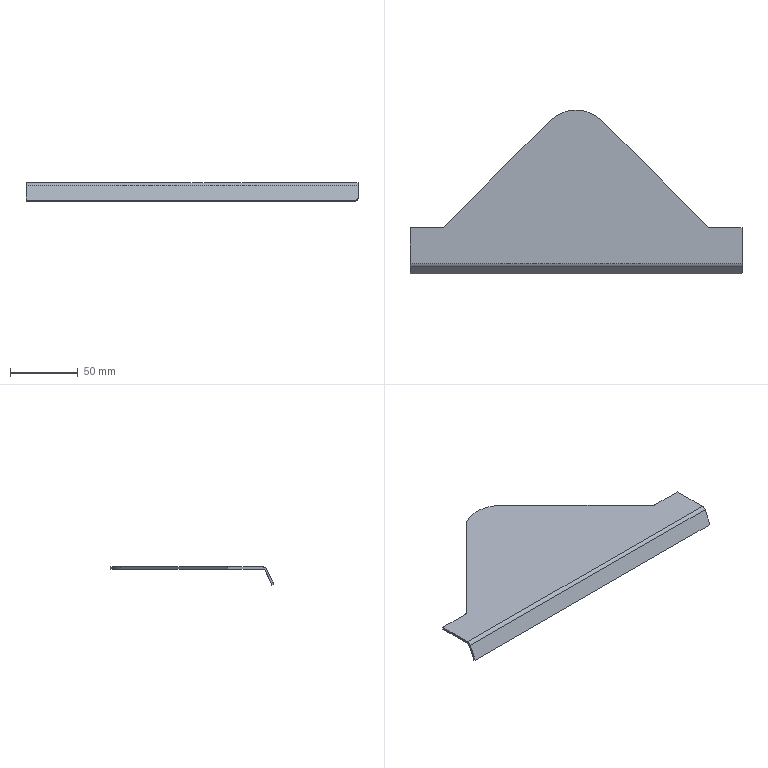Part | STEP file | Guard wheel drive wer2 part2 | 1 solid | 21 faces | box 245 x 120.904 x 13.322 mm | volume 29188 mm3 | plane 15 | cylinder 6 | commonest cylinder face diameters 3 x3 4 x1 6 x1 54 x1
STEP:
#1=CARTESIAN_POINT('',(0.,0.,0.));
#2=DIRECTION('',(0.,0.,1.));
#3=DIRECTION('',(1.,0.,0.));
#4=AXIS2_PLACEMENT_3D('',#1,#2,#3);
#5=CARTESIAN_POINT('',(221.305,-31.558,-9.376));
#6=VERTEX_POINT('',#5);
#7=CARTESIAN_POINT('',(219.305,-32.404,-11.188));
#8=VERTEX_POINT('',#7);
#9=CARTESIAN_POINT('',(219.305,-31.558,-9.376));
#10=DIRECTION('',(0.,0.9063,-0.4226));
#11=DIRECTION('',(0.7071,-0.2988,-0.6409));
#12=AXIS2_PLACEMENT_3D('',#9,#10,#11);
#13=CIRCLE('',#12,2.);
#14=CARTESIAN_POINT('',(219.305,-30.199,-10.01));
#15=DIRECTION('',(0.,-0.9063,0.4226));
#16=DIRECTION('',(0.7071,-0.2988,-0.6409));
#17=AXIS2_PLACEMENT_3D('',#14,#15,#16);
#18=CYLINDRICAL_SURFACE('',#17,2.);
#19=CARTESIAN_POINT('',(12.566,1.5));
#20=DIRECTION('',(-1.,0.));
#21=VECTOR('',#20,1.);
#22=LINE('',#19,#21);
#23=(GEOMETRIC_REPRESENTATION_CONTEXT(2)PARAMETRIC_REPRESENTATION_CONTEXT()REPRESENTATION_CONTEXT('',''));
#24=DEFINITIONAL_REPRESENTATION('',(#22),#23);
#25=PCURVE('',#18,#24);
#26=CARTESIAN_POINT('',(98.805,-29.331,-4.6));
#27=DIRECTION('',(0.,-0.9063,0.4226));
#28=DIRECTION('',(1.,0.,0.));
#29=AXIS2_PLACEMENT_3D('',#26,#27,#28);
#30=PLANE('',#29);
#31=CARTESIAN_POINT('',(121.914,-6.684));
#32=CARTESIAN_POINT('',(119.465,-9.133));
#33=CARTESIAN_POINT('',(118.568,-5.787));
#34=CARTESIAN_POINT('',(117.672,-2.441));
#35=CARTESIAN_POINT('',(121.018,-3.338));
#36=CARTESIAN_POINT('',(124.364,-4.234));
#37=CARTESIAN_POINT('',(121.914,-6.684));
#38=(BOUNDED_CURVE()B_SPLINE_CURVE(2,(#31,#32,#33,#34,#35,#36,#37),.UNSPECIFIED.,.T.,.F.)B_SPLINE_CURVE_WITH_KNOTS((1,2,2,2,2,1),(-2.094,0.,2.094,4.189,6.283,8.378),.UNSPECIFIED.)CURVE()GEOMETRIC_REPRESENTATION_ITEM()RATIONAL_B_SPLINE_CURVE((1.,0.5,1.,0.5,1.,0.5,1.))REPRESENTATION_ITEM(''));
#39=(GEOMETRIC_REPRESENTATION_CONTEXT(2)PARAMETRIC_REPRESENTATION_CONTEXT()REPRESENTATION_CONTEXT('',''));
#40=DEFINITIONAL_REPRESENTATION('',(#38),#39);
#41=PCURVE('',#30,#40);
#42=SURFACE_CURVE('',#13,(#25,#41),.PCURVE_S1.);
#43=EDGE_CURVE('',#6,#8,#42,.T.);
#44=ORIENTED_EDGE('',*,*,#43,.T.);
#45=CARTESIAN_POINT('',(219.305,-31.044,-11.822));
#46=VERTEX_POINT('',#45);
#47=CARTESIAN_POINT('',(219.305,-31.044,-11.822));
#48=DIRECTION('',(0.,0.9063,-0.4226));
#49=VECTOR('',#48,1.);
#50=LINE('',#47,#49);
#51=CARTESIAN_POINT('',(5.498,0.));
#52=DIRECTION('',(0.,-1.));
#53=VECTOR('',#52,1.);
#54=LINE('',#51,#53);
#55=(GEOMETRIC_REPRESENTATION_CONTEXT(2)PARAMETRIC_REPRESENTATION_CONTEXT()REPRESENTATION_CONTEXT('',''));
#56=DEFINITIONAL_REPRESENTATION('',(#54),#55);
#57=PCURVE('',#18,#56);
#58=CARTESIAN_POINT('',(221.305,-31.044,-11.822));
#59=DIRECTION('',(0.,-0.4226,-0.9063));
#60=DIRECTION('',(0.,0.9063,-0.4226));
#61=AXIS2_PLACEMENT_3D('',#58,#59,#60);
#62=PLANE('',#61);
#63=CARTESIAN_POINT('',(0.,-2.));
#64=DIRECTION('',(1.,0.));
#65=VECTOR('',#64,1.);
#66=LINE('',#63,#65);
#67=(GEOMETRIC_REPRESENTATION_CONTEXT(2)PARAMETRIC_REPRESENTATION_CONTEXT()REPRESENTATION_CONTEXT('',''));
#68=DEFINITIONAL_REPRESENTATION('',(#66),#67);
#69=PCURVE('',#62,#68);
#70=SURFACE_CURVE('',#50,(#57,#69),.PCURVE_S1.);
#71=EDGE_CURVE('',#8,#46,#70,.T.);
#72=ORIENTED_EDGE('',*,*,#71,.T.);
#73=CARTESIAN_POINT('',(221.305,-30.199,-10.01));
#74=VERTEX_POINT('',#73);
#75=CARTESIAN_POINT('',(219.305,-30.199,-10.01));
#76=DIRECTION('',(0.,-0.9063,0.4226));
#77=DIRECTION('',(0.7071,-0.2988,-0.6409));
#78=AXIS2_PLACEMENT_3D('',#75,#76,#77);
#79=CIRCLE('',#78,2.);
#80=CARTESIAN_POINT('',(0.,0.));
#81=DIRECTION('',(1.,0.));
#82=VECTOR('',#81,1.);
#83=LINE('',#80,#82);
#84=(GEOMETRIC_REPRESENTATION_CONTEXT(2)PARAMETRIC_REPRESENTATION_CONTEXT()REPRESENTATION_CONTEXT('',''));
#85=DEFINITIONAL_REPRESENTATION('',(#83),#84);
#86=PCURVE('',#18,#85);
#87=CARTESIAN_POINT('',(98.805,-27.972,-5.234));
#88=DIRECTION('',(0.,-0.9063,0.4226));
#89=DIRECTION('',(1.,0.,0.));
#90=AXIS2_PLACEMENT_3D('',#87,#88,#89);
#91=PLANE('',#90);
#92=CARTESIAN_POINT('',(120.5,-5.27));
#93=DIRECTION('',(0.7071,-0.7071));
#94=AXIS2_PLACEMENT_2D('',#92,#93);
#95=CIRCLE('',#94,2.);
#96=(GEOMETRIC_REPRESENTATION_CONTEXT(2)PARAMETRIC_REPRESENTATION_CONTEXT()REPRESENTATION_CONTEXT('',''));
#97=DEFINITIONAL_REPRESENTATION('',(#95),#96);
#98=PCURVE('',#91,#97);
#99=SURFACE_CURVE('',#79,(#86,#98),.PCURVE_S1.);
#100=EDGE_CURVE('',#46,#74,#99,.T.);
#101=ORIENTED_EDGE('',*,*,#100,.T.);
#102=CARTESIAN_POINT('',(221.305,-30.199,-10.01));
#103=DIRECTION('',(0.,-0.9063,0.4226));
#104=VECTOR('',#103,1.);
#105=LINE('',#102,#104);
#106=CARTESIAN_POINT('',(7.069,0.));
#107=DIRECTION('',(0.,1.));
#108=VECTOR('',#107,1.);
#109=LINE('',#106,#108);
#110=(GEOMETRIC_REPRESENTATION_CONTEXT(2)PARAMETRIC_REPRESENTATION_CONTEXT()REPRESENTATION_CONTEXT('',''));
#111=DEFINITIONAL_REPRESENTATION('',(#109),#110);
#112=PCURVE('',#18,#111);
#113=CARTESIAN_POINT('',(221.305,-25.935,-0.8661));
#114=DIRECTION('',(1.,0.,0.));
#115=DIRECTION('',(0.,0.9063,-0.4226));
#116=AXIS2_PLACEMENT_3D('',#113,#114,#115);
#117=PLANE('',#116);
#118=CARTESIAN_POINT('',(0.,-10.089));
#119=DIRECTION('',(-1.,0.));
#120=VECTOR('',#119,1.);
#121=LINE('',#118,#120);
#122=(GEOMETRIC_REPRESENTATION_CONTEXT(2)PARAMETRIC_REPRESENTATION_CONTEXT()REPRESENTATION_CONTEXT('',''));
#123=DEFINITIONAL_REPRESENTATION('',(#121),#122);
#124=PCURVE('',#117,#123);
#125=SURFACE_CURVE('',#105,(#112,#124),.PCURVE_S1.);
#126=EDGE_CURVE('',#74,#6,#125,.T.);
#127=ORIENTED_EDGE('',*,*,#126,.T.);
#128=EDGE_LOOP('',(#44,#72,#101,#127));
#129=FACE_BOUND('',#128,.T.);
#130=ADVANCED_FACE('',(#129),#18,.T.);
#131=ORIENTED_EDGE('',*,*,#126,.F.);
#132=CARTESIAN_POINT('',(221.305,-25.935,-0.8661));
#133=VERTEX_POINT('',#132);
#134=CARTESIAN_POINT('',(221.305,-23.067,5.284));
#135=DIRECTION('',(0.,0.4226,0.9063));
#136=VECTOR('',#135,1.);
#137=LINE('',#134,#136);
#138=CARTESIAN_POINT('',(0.,6.786));
#139=DIRECTION('',(0.,1.));
#140=VECTOR('',#139,1.);
#141=LINE('',#138,#140);
#142=(GEOMETRIC_REPRESENTATION_CONTEXT(2)PARAMETRIC_REPRESENTATION_CONTEXT()REPRESENTATION_CONTEXT('',''));
#143=DEFINITIONAL_REPRESENTATION('',(#141),#142);
#144=PCURVE('',#117,#143);
#145=CARTESIAN_POINT('',(122.5,11.605));
#146=DIRECTION('',(0.,1.));
#147=VECTOR('',#146,1.);
#148=LINE('',#145,#147);
#149=(GEOMETRIC_REPRESENTATION_CONTEXT(2)PARAMETRIC_REPRESENTATION_CONTEXT()REPRESENTATION_CONTEXT('',''));
#150=DEFINITIONAL_REPRESENTATION('',(#148),#149);
#151=PCURVE('',#91,#150);
#152=SURFACE_CURVE('',#137,(#144,#151),.PCURVE_S1.);
#153=EDGE_CURVE('',#74,#133,#152,.T.);
#154=ORIENTED_EDGE('',*,*,#153,.T.);
#155=CARTESIAN_POINT('',(221.305,-27.295,-0.2321));
#156=VERTEX_POINT('',#155);
#157=CARTESIAN_POINT('',(221.305,-26.234,-0.7266));
#158=DIRECTION('',(0.,-0.9063,0.4226));
#159=VECTOR('',#158,1.);
#160=LINE('',#157,#159);
#161=CARTESIAN_POINT('',(-0.33,0.));
#162=DIRECTION('',(-1.,0.));
#163=VECTOR('',#162,1.);
#164=LINE('',#161,#163);
#165=(GEOMETRIC_REPRESENTATION_CONTEXT(2)PARAMETRIC_REPRESENTATION_CONTEXT()REPRESENTATION_CONTEXT('',''));
#166=DEFINITIONAL_REPRESENTATION('',(#164),#165);
#167=PCURVE('',#117,#166);
#168=CARTESIAN_POINT('',(221.305,-25.935,-0.8661));
#169=DIRECTION('',(1.,0.,0.));
#170=DIRECTION('',(0.,0.,-1.));
#171=AXIS2_PLACEMENT_3D('',#168,#169,#170);
#172=PLANE('',#171);
#173=CARTESIAN_POINT('',(-0.1395,-0.2991));
#174=DIRECTION('',(-0.4226,-0.9063));
#175=VECTOR('',#174,1.);
#176=LINE('',#173,#175);
#177=(GEOMETRIC_REPRESENTATION_CONTEXT(2)PARAMETRIC_REPRESENTATION_CONTEXT()REPRESENTATION_CONTEXT('',''));
#178=DEFINITIONAL_REPRESENTATION('',(#176),#177);
#179=PCURVE('',#172,#178);
#180=SURFACE_CURVE('',#160,(#167,#179),.PCURVE_S1.);
#181=EDGE_CURVE('',#133,#156,#180,.T.);
#182=ORIENTED_EDGE('',*,*,#181,.T.);
#183=CARTESIAN_POINT('',(221.305,-27.295,-0.2321));
#184=DIRECTION('',(0.,-0.4226,-0.9063));
#185=VECTOR('',#184,1.);
#186=LINE('',#183,#185);
#187=CARTESIAN_POINT('',(-1.5,0.));
#188=DIRECTION('',(0.,-1.));
#189=VECTOR('',#188,1.);
#190=LINE('',#187,#189);
#191=(GEOMETRIC_REPRESENTATION_CONTEXT(2)PARAMETRIC_REPRESENTATION_CONTEXT()REPRESENTATION_CONTEXT('',''));
#192=DEFINITIONAL_REPRESENTATION('',(#190),#191);
#193=PCURVE('',#117,#192);
#194=CARTESIAN_POINT('',(122.5,4.819));
#195=DIRECTION('',(0.,-1.));
#196=VECTOR('',#195,1.);
#197=LINE('',#194,#196);
#198=(GEOMETRIC_REPRESENTATION_CONTEXT(2)PARAMETRIC_REPRESENTATION_CONTEXT()REPRESENTATION_CONTEXT('',''));
#199=DEFINITIONAL_REPRESENTATION('',(#197),#198);
#200=PCURVE('',#30,#199);
#201=SURFACE_CURVE('',#186,(#193,#200),.PCURVE_S1.);
#202=EDGE_CURVE('',#156,#6,#201,.T.);
#203=ORIENTED_EDGE('',*,*,#202,.T.);
#204=EDGE_LOOP('',(#131,#154,#182,#203));
#205=FACE_BOUND('',#204,.T.);
#206=ADVANCED_FACE('',(#205),#117,.T.);
#207=ORIENTED_EDGE('',*,*,#100,.F.);
#208=CARTESIAN_POINT('',(-23.695,-31.044,-11.822));
#209=VERTEX_POINT('',#208);
#210=CARTESIAN_POINT('',(221.305,-31.044,-11.822));
#211=DIRECTION('',(-1.,0.,0.));
#212=VECTOR('',#211,1.);
#213=LINE('',#210,#212);
#214=CARTESIAN_POINT('',(122.5,-7.27));
#215=DIRECTION('',(-1.,0.));
#216=VECTOR('',#215,1.);
#217=LINE('',#214,#216);
#218=(GEOMETRIC_REPRESENTATION_CONTEXT(2)PARAMETRIC_REPRESENTATION_CONTEXT()REPRESENTATION_CONTEXT('',''));
#219=DEFINITIONAL_REPRESENTATION('',(#217),#218);
#220=PCURVE('',#91,#219);
#221=CARTESIAN_POINT('',(0.,0.));
#222=DIRECTION('',(0.,-1.));
#223=VECTOR('',#222,1.);
#224=LINE('',#221,#223);
#225=(GEOMETRIC_REPRESENTATION_CONTEXT(2)PARAMETRIC_REPRESENTATION_CONTEXT()REPRESENTATION_CONTEXT('',''));
#226=DEFINITIONAL_REPRESENTATION('',(#224),#225);
#227=PCURVE('',#62,#226);
#228=SURFACE_CURVE('',#213,(#220,#227),.PCURVE_S1.);
#229=EDGE_CURVE('',#46,#209,#228,.T.);
#230=ORIENTED_EDGE('',*,*,#229,.T.);
#231=CARTESIAN_POINT('',(-23.695,-25.935,-0.8661));
#232=VERTEX_POINT('',#231);
#233=CARTESIAN_POINT('',(-23.695,-23.067,5.284));
#234=DIRECTION('',(0.,0.4226,0.9063));
#235=VECTOR('',#234,1.);
#236=LINE('',#233,#235);
#237=CARTESIAN_POINT('',(-122.5,11.605));
#238=DIRECTION('',(0.,1.));
#239=VECTOR('',#238,1.);
#240=LINE('',#237,#239);
#241=(GEOMETRIC_REPRESENTATION_CONTEXT(2)PARAMETRIC_REPRESENTATION_CONTEXT()REPRESENTATION_CONTEXT('',''));
#242=DEFINITIONAL_REPRESENTATION('',(#240),#241);
#243=PCURVE('',#91,#242);
#244=CARTESIAN_POINT('',(-23.695,-25.935,-0.8661));
#245=DIRECTION('',(-1.,0.,0.));
#246=DIRECTION('',(0.,-0.9063,0.4226));
#247=AXIS2_PLACEMENT_3D('',#244,#245,#246);
#248=PLANE('',#247);
#249=CARTESIAN_POINT('',(0.,6.786));
#250=DIRECTION('',(0.,1.));
#251=VECTOR('',#250,1.);
#252=LINE('',#249,#251);
#253=(GEOMETRIC_REPRESENTATION_CONTEXT(2)PARAMETRIC_REPRESENTATION_CONTEXT()REPRESENTATION_CONTEXT('',''));
#254=DEFINITIONAL_REPRESENTATION('',(#252),#253);
#255=PCURVE('',#248,#254);
#256=SURFACE_CURVE('',#236,(#243,#255),.PCURVE_S1.);
#257=EDGE_CURVE('',#209,#232,#256,.T.);
#258=ORIENTED_EDGE('',*,*,#257,.T.);
#259=CARTESIAN_POINT('',(98.805,-25.935,-0.8661));
#260=DIRECTION('',(1.,0.,0.));
#261=VECTOR('',#260,1.);
#262=LINE('',#259,#261);
#263=CARTESIAN_POINT('',(0.,4.819));
#264=DIRECTION('',(1.,0.));
#265=VECTOR('',#264,1.);
#266=LINE('',#263,#265);
#267=(GEOMETRIC_REPRESENTATION_CONTEXT(2)PARAMETRIC_REPRESENTATION_CONTEXT()REPRESENTATION_CONTEXT('',''));
#268=DEFINITIONAL_REPRESENTATION('',(#266),#267);
#269=PCURVE('',#91,#268);
#270=CARTESIAN_POINT('',(98.805,-24.576,-1.5));
#271=DIRECTION('',(1.,0.,0.));
#272=DIRECTION('',(0.,0.,1.));
#273=AXIS2_PLACEMENT_3D('',#270,#271,#272);
#274=CYLINDRICAL_SURFACE('',#273,1.5);
#275=CARTESIAN_POINT('',(1.134,0.));
#276=DIRECTION('',(0.,1.));
#277=VECTOR('',#276,1.);
#278=LINE('',#275,#277);
#279=(GEOMETRIC_REPRESENTATION_CONTEXT(2)PARAMETRIC_REPRESENTATION_CONTEXT()REPRESENTATION_CONTEXT('',''));
#280=DEFINITIONAL_REPRESENTATION('',(#278),#279);
#281=PCURVE('',#274,#280);
#282=SURFACE_CURVE('',#262,(#269,#281),.PCURVE_S1.);
#283=EDGE_CURVE('',#232,#133,#282,.T.);
#284=ORIENTED_EDGE('',*,*,#283,.T.);
#285=ORIENTED_EDGE('',*,*,#153,.F.);
#286=EDGE_LOOP('',(#207,#230,#258,#284,#285));
#287=FACE_BOUND('',#286,.T.);
#288=ADVANCED_FACE('',(#287),#91,.F.);
#289=CARTESIAN_POINT('',(-23.695,-27.295,-0.2321));
#290=VERTEX_POINT('',#289);
#291=CARTESIAN_POINT('',(98.805,-27.295,-0.2321));
#292=DIRECTION('',(-1.,0.,0.));
#293=VECTOR('',#292,1.);
#294=LINE('',#291,#293);
#295=CARTESIAN_POINT('',(98.805,-24.576,-1.5));
#296=DIRECTION('',(1.,0.,0.));
#297=DIRECTION('',(0.,0.,1.));
#298=AXIS2_PLACEMENT_3D('',#295,#296,#297);
#299=CYLINDRICAL_SURFACE('',#298,3.);
#300=CARTESIAN_POINT('',(1.134,0.));
#301=DIRECTION('',(0.,-1.));
#302=VECTOR('',#301,1.);
#303=LINE('',#300,#302);
#304=(GEOMETRIC_REPRESENTATION_CONTEXT(2)PARAMETRIC_REPRESENTATION_CONTEXT()REPRESENTATION_CONTEXT('',''));
#305=DEFINITIONAL_REPRESENTATION('',(#303),#304);
#306=PCURVE('',#299,#305);
#307=CARTESIAN_POINT('',(0.,4.819));
#308=DIRECTION('',(-1.,0.));
#309=VECTOR('',#308,1.);
#310=LINE('',#307,#309);
#311=(GEOMETRIC_REPRESENTATION_CONTEXT(2)PARAMETRIC_REPRESENTATION_CONTEXT()REPRESENTATION_CONTEXT('',''));
#312=DEFINITIONAL_REPRESENTATION('',(#310),#311);
#313=PCURVE('',#30,#312);
#314=SURFACE_CURVE('',#294,(#306,#313),.PCURVE_S1.);
#315=EDGE_CURVE('',#156,#290,#314,.T.);
#316=ORIENTED_EDGE('',*,*,#315,.F.);
#317=CARTESIAN_POINT('',(221.305,-24.576,1.5));
#318=VERTEX_POINT('',#317);
#319=CARTESIAN_POINT('',(221.305,-24.576,-1.5));
#320=DIRECTION('',(1.,0.,0.));
#321=DIRECTION('',(0.,0.,1.));
#322=AXIS2_PLACEMENT_3D('',#319,#320,#321);
#323=CIRCLE('',#322,3.);
#324=CARTESIAN_POINT('',(0.,122.5));
#325=DIRECTION('',(1.,0.));
#326=VECTOR('',#325,1.);
#327=LINE('',#324,#326);
#328=(GEOMETRIC_REPRESENTATION_CONTEXT(2)PARAMETRIC_REPRESENTATION_CONTEXT()REPRESENTATION_CONTEXT('',''));
#329=DEFINITIONAL_REPRESENTATION('',(#327),#328);
#330=PCURVE('',#299,#329);
#331=CARTESIAN_POINT('',(0.6339,1.359));
#332=DIRECTION('',(-1.,0.));
#333=AXIS2_PLACEMENT_2D('',#331,#332);
#334=CIRCLE('',#333,3.);
#335=(GEOMETRIC_REPRESENTATION_CONTEXT(2)PARAMETRIC_REPRESENTATION_CONTEXT()REPRESENTATION_CONTEXT('',''));
#336=DEFINITIONAL_REPRESENTATION('',(#334),#335);
#337=PCURVE('',#172,#336);
#338=SURFACE_CURVE('',#323,(#330,#337),.PCURVE_S1.);
#339=EDGE_CURVE('',#318,#156,#338,.T.);
#340=ORIENTED_EDGE('',*,*,#339,.F.);
#341=CARTESIAN_POINT('',(-23.695,-24.576,1.5));
#342=VERTEX_POINT('',#341);
#343=CARTESIAN_POINT('',(86.524,-24.576,1.5));
#344=DIRECTION('',(1.,0.,0.));
#345=VECTOR('',#344,1.);
#346=LINE('',#343,#345);
#347=CARTESIAN_POINT('',(0.,-12.281));
#348=DIRECTION('',(0.,1.));
#349=VECTOR('',#348,1.);
#350=LINE('',#347,#349);
#351=(GEOMETRIC_REPRESENTATION_CONTEXT(2)PARAMETRIC_REPRESENTATION_CONTEXT()REPRESENTATION_CONTEXT('',''));
#352=DEFINITIONAL_REPRESENTATION('',(#350),#351);
#353=PCURVE('',#299,#352);
#354=CARTESIAN_POINT('',(196.743,0.9072,1.5));
#355=DIRECTION('',(0.,0.,1.));
#356=DIRECTION('',(1.,0.,0.));
#357=AXIS2_PLACEMENT_3D('',#354,#355,#356);
#358=PLANE('',#357);
#359=CARTESIAN_POINT('',(-110.219,-25.483));
#360=DIRECTION('',(1.,0.));
#361=VECTOR('',#360,1.);
#362=LINE('',#359,#361);
#363=(GEOMETRIC_REPRESENTATION_CONTEXT(2)PARAMETRIC_REPRESENTATION_CONTEXT()REPRESENTATION_CONTEXT('',''));
#364=DEFINITIONAL_REPRESENTATION('',(#362),#363);
#365=PCURVE('',#358,#364);
#366=SURFACE_CURVE('',#346,(#353,#365),.PCURVE_S1.);
#367=EDGE_CURVE('',#342,#318,#366,.T.);
#368=ORIENTED_EDGE('',*,*,#367,.F.);
#369=CARTESIAN_POINT('',(-23.695,-24.576,-1.5));
#370=DIRECTION('',(-1.,0.,0.));
#371=DIRECTION('',(0.,-0.9063,0.4226));
#372=AXIS2_PLACEMENT_3D('',#369,#370,#371);
#373=CIRCLE('',#372,3.);
#374=CARTESIAN_POINT('',(1.134,-122.5));
#375=DIRECTION('',(-1.,0.));
#376=VECTOR('',#375,1.);
#377=LINE('',#374,#376);
#378=(GEOMETRIC_REPRESENTATION_CONTEXT(2)PARAMETRIC_REPRESENTATION_CONTEXT()REPRESENTATION_CONTEXT('',''));
#379=DEFINITIONAL_REPRESENTATION('',(#377),#378);
#380=PCURVE('',#299,#379);
#381=CARTESIAN_POINT('',(-23.695,-27.295,-0.2321));
#382=DIRECTION('',(-1.,0.,0.));
#383=DIRECTION('',(0.,0.,1.));
#384=AXIS2_PLACEMENT_3D('',#381,#382,#383);
#385=PLANE('',#384);
#386=CARTESIAN_POINT('',(-1.268,2.719));
#387=DIRECTION('',(0.4226,-0.9063));
#388=AXIS2_PLACEMENT_2D('',#386,#387);
#389=CIRCLE('',#388,3.);
#390=(GEOMETRIC_REPRESENTATION_CONTEXT(2)PARAMETRIC_REPRESENTATION_CONTEXT()REPRESENTATION_CONTEXT('',''));
#391=DEFINITIONAL_REPRESENTATION('',(#389),#390);
#392=PCURVE('',#385,#391);
#393=SURFACE_CURVE('',#373,(#380,#392),.PCURVE_S1.);
#394=EDGE_CURVE('',#290,#342,#393,.T.);
#395=ORIENTED_EDGE('',*,*,#394,.F.);
#396=EDGE_LOOP('',(#316,#340,#368,#395));
#397=FACE_BOUND('',#396,.T.);
#398=ADVANCED_FACE('',(#397),#299,.T.);
#399=CARTESIAN_POINT('',(-23.695,-26.234,-0.7266));
#400=DIRECTION('',(0.,0.9063,-0.4226));
#401=VECTOR('',#400,1.);
#402=LINE('',#399,#401);
#403=CARTESIAN_POINT('',(0.33,0.));
#404=DIRECTION('',(-1.,0.));
#405=VECTOR('',#404,1.);
#406=LINE('',#403,#405);
#407=(GEOMETRIC_REPRESENTATION_CONTEXT(2)PARAMETRIC_REPRESENTATION_CONTEXT()REPRESENTATION_CONTEXT('',''));
#408=DEFINITIONAL_REPRESENTATION('',(#406),#407);
#409=PCURVE('',#248,#408);
#410=CARTESIAN_POINT('',(-0.4945,1.06));
#411=DIRECTION('',(-0.4226,0.9063));
#412=VECTOR('',#411,1.);
#413=LINE('',#410,#412);
#414=(GEOMETRIC_REPRESENTATION_CONTEXT(2)PARAMETRIC_REPRESENTATION_CONTEXT()REPRESENTATION_CONTEXT('',''));
#415=DEFINITIONAL_REPRESENTATION('',(#413),#414);
#416=PCURVE('',#385,#415);
#417=SURFACE_CURVE('',#402,(#409,#416),.PCURVE_S1.);
#418=EDGE_CURVE('',#290,#232,#417,.T.);
#419=ORIENTED_EDGE('',*,*,#418,.T.);
#420=ORIENTED_EDGE('',*,*,#257,.F.);
#421=CARTESIAN_POINT('',(-23.695,-32.404,-11.188));
#422=VERTEX_POINT('',#421);
#423=CARTESIAN_POINT('',(-23.695,-31.044,-11.822));
#424=DIRECTION('',(0.,-0.9063,0.4226));
#425=VECTOR('',#424,1.);
#426=LINE('',#423,#425);
#427=CARTESIAN_POINT('',(0.,-12.089));
#428=DIRECTION('',(1.,0.));
#429=VECTOR('',#428,1.);
#430=LINE('',#427,#429);
#431=(GEOMETRIC_REPRESENTATION_CONTEXT(2)PARAMETRIC_REPRESENTATION_CONTEXT()REPRESENTATION_CONTEXT('',''));
#432=DEFINITIONAL_REPRESENTATION('',(#430),#431);
#433=PCURVE('',#248,#432);
#434=CARTESIAN_POINT('',(0.,-245.));
#435=DIRECTION('',(-1.,0.));
#436=VECTOR('',#435,1.);
#437=LINE('',#434,#436);
#438=(GEOMETRIC_REPRESENTATION_CONTEXT(2)PARAMETRIC_REPRESENTATION_CONTEXT()REPRESENTATION_CONTEXT('',''));
#439=DEFINITIONAL_REPRESENTATION('',(#437),#438);
#440=PCURVE('',#62,#439);
#441=SURFACE_CURVE('',#426,(#433,#440),.PCURVE_S1.);
#442=EDGE_CURVE('',#209,#422,#441,.T.);
#443=ORIENTED_EDGE('',*,*,#442,.T.);
#444=CARTESIAN_POINT('',(-23.695,-24.427,5.918));
#445=DIRECTION('',(0.,0.4226,0.9063));
#446=VECTOR('',#445,1.);
#447=LINE('',#444,#446);
#448=CARTESIAN_POINT('',(1.5,6.786));
#449=DIRECTION('',(0.,1.));
#450=VECTOR('',#449,1.);
#451=LINE('',#448,#450);
#452=(GEOMETRIC_REPRESENTATION_CONTEXT(2)PARAMETRIC_REPRESENTATION_CONTEXT()REPRESENTATION_CONTEXT('',''));
#453=DEFINITIONAL_REPRESENTATION('',(#451),#452);
#454=PCURVE('',#248,#453);
#455=CARTESIAN_POINT('',(-122.5,11.605));
#456=DIRECTION('',(0.,1.));
#457=VECTOR('',#456,1.);
#458=LINE('',#455,#457);
#459=(GEOMETRIC_REPRESENTATION_CONTEXT(2)PARAMETRIC_REPRESENTATION_CONTEXT()REPRESENTATION_CONTEXT('',''));
#460=DEFINITIONAL_REPRESENTATION('',(#458),#459);
#461=PCURVE('',#30,#460);
#462=SURFACE_CURVE('',#447,(#454,#461),.PCURVE_S1.);
#463=EDGE_CURVE('',#422,#290,#462,.T.);
#464=ORIENTED_EDGE('',*,*,#463,.T.);
#465=EDGE_LOOP('',(#419,#420,#443,#464));
#466=FACE_BOUND('',#465,.T.);
#467=ADVANCED_FACE('',(#466),#248,.T.);
#468=ORIENTED_EDGE('',*,*,#181,.F.);
#469=CARTESIAN_POINT('',(221.305,-24.576,0.));
#470=VERTEX_POINT('',#469);
#471=CARTESIAN_POINT('',(221.305,-24.576,-1.5));
#472=DIRECTION('',(-1.,0.,0.));
#473=DIRECTION('',(0.,-0.9063,0.4226));
#474=AXIS2_PLACEMENT_3D('',#471,#472,#473);
#475=CIRCLE('',#474,1.5);
#476=CARTESIAN_POINT('',(0.,0.));
#477=CARTESIAN_POINT('',(-2.355,1.098));
#478=CARTESIAN_POINT('',(-0.2264,2.588));
#479=CARTESIAN_POINT('',(1.902,4.078));
#480=CARTESIAN_POINT('',(2.128,1.49));
#481=CARTESIAN_POINT('',(2.355,-1.098));
#482=CARTESIAN_POINT('',(0.,0.));
#483=(BOUNDED_CURVE()B_SPLINE_CURVE(2,(#476,#477,#478,#479,#480,#481,#482),.UNSPECIFIED.,.T.,.F.)B_SPLINE_CURVE_WITH_KNOTS((1,2,2,2,2,1),(-2.094,0.,2.094,4.189,6.283,8.378),.UNSPECIFIED.)CURVE()GEOMETRIC_REPRESENTATION_ITEM()RATIONAL_B_SPLINE_CURVE((1.,0.5,1.,0.5,1.,0.5,1.))REPRESENTATION_ITEM(''));
#484=(GEOMETRIC_REPRESENTATION_CONTEXT(2)PARAMETRIC_REPRESENTATION_CONTEXT()REPRESENTATION_CONTEXT('',''));
#485=DEFINITIONAL_REPRESENTATION('',(#483),#484);
#486=PCURVE('',#172,#485);
#487=CARTESIAN_POINT('',(1.134,122.5));
#488=DIRECTION('',(-1.,0.));
#489=VECTOR('',#488,1.);
#490=LINE('',#487,#489);
#491=(GEOMETRIC_REPRESENTATION_CONTEXT(2)PARAMETRIC_REPRESENTATION_CONTEXT()REPRESENTATION_CONTEXT('',''));
#492=DEFINITIONAL_REPRESENTATION('',(#490),#491);
#493=PCURVE('',#274,#492);
#494=SURFACE_CURVE('',#475,(#486,#493),.PCURVE_S1.);
#495=EDGE_CURVE('',#133,#470,#494,.T.);
#496=ORIENTED_EDGE('',*,*,#495,.T.);
#497=CARTESIAN_POINT('',(221.305,-24.576,0.));
#498=DIRECTION('',(0.,0.,-1.));
#499=VECTOR('',#498,1.);
#500=LINE('',#497,#499);
#501=CARTESIAN_POINT('',(-0.8661,1.359));
#502=DIRECTION('',(1.,0.));
#503=VECTOR('',#502,1.);
#504=LINE('',#501,#503);
#505=(GEOMETRIC_REPRESENTATION_CONTEXT(2)PARAMETRIC_REPRESENTATION_CONTEXT()REPRESENTATION_CONTEXT('',''));
#506=DEFINITIONAL_REPRESENTATION('',(#504),#505);
#507=PCURVE('',#172,#506);
#508=CARTESIAN_POINT('',(221.305,1.5,0.));
#509=DIRECTION('',(1.,0.,0.));
#510=DIRECTION('',(0.,0.,-1.));
#511=AXIS2_PLACEMENT_3D('',#508,#509,#510);
#512=PLANE('',#511);
#513=CARTESIAN_POINT('',(0.,-26.076));
#514=DIRECTION('',(1.,0.));
#515=VECTOR('',#514,1.);
#516=LINE('',#513,#515);
#517=(GEOMETRIC_REPRESENTATION_CONTEXT(2)PARAMETRIC_REPRESENTATION_CONTEXT()REPRESENTATION_CONTEXT('',''));
#518=DEFINITIONAL_REPRESENTATION('',(#516),#517);
#519=PCURVE('',#512,#518);
#520=SURFACE_CURVE('',#500,(#507,#519),.PCURVE_S1.);
#521=EDGE_CURVE('',#318,#470,#520,.T.);
#522=ORIENTED_EDGE('',*,*,#521,.F.);
#523=ORIENTED_EDGE('',*,*,#339,.T.);
#524=EDGE_LOOP('',(#468,#496,#522,#523));
#525=FACE_BOUND('',#524,.T.);
#526=ADVANCED_FACE('',(#525),#172,.T.);
#527=ORIENTED_EDGE('',*,*,#418,.F.);
#528=ORIENTED_EDGE('',*,*,#394,.T.);
#529=CARTESIAN_POINT('',(-23.695,-24.576,0.));
#530=VERTEX_POINT('',#529);
#531=CARTESIAN_POINT('',(-23.695,-24.576,0.));
#532=DIRECTION('',(0.,0.,1.));
#533=VECTOR('',#532,1.);
#534=LINE('',#531,#533);
#535=CARTESIAN_POINT('',(0.2321,2.719));
#536=DIRECTION('',(1.,0.));
#537=VECTOR('',#536,1.);
#538=LINE('',#535,#537);
#539=(GEOMETRIC_REPRESENTATION_CONTEXT(2)PARAMETRIC_REPRESENTATION_CONTEXT()REPRESENTATION_CONTEXT('',''));
#540=DEFINITIONAL_REPRESENTATION('',(#538),#539);
#541=PCURVE('',#385,#540);
#542=CARTESIAN_POINT('',(-23.695,-26.487,0.));
#543=DIRECTION('',(-1.,0.,0.));
#544=DIRECTION('',(0.,0.,1.));
#545=AXIS2_PLACEMENT_3D('',#542,#543,#544);
#546=PLANE('',#545);
#547=CARTESIAN_POINT('',(0.,1.911));
#548=DIRECTION('',(1.,0.));
#549=VECTOR('',#548,1.);
#550=LINE('',#547,#549);
#551=(GEOMETRIC_REPRESENTATION_CONTEXT(2)PARAMETRIC_REPRESENTATION_CONTEXT()REPRESENTATION_CONTEXT('',''));
#552=DEFINITIONAL_REPRESENTATION('',(#550),#551);
#553=PCURVE('',#546,#552);
#554=SURFACE_CURVE('',#534,(#541,#553),.PCURVE_S1.);
#555=EDGE_CURVE('',#530,#342,#554,.T.);
#556=ORIENTED_EDGE('',*,*,#555,.F.);
#557=CARTESIAN_POINT('',(-23.695,-24.576,-1.5));
#558=DIRECTION('',(-1.,0.,0.));
#559=DIRECTION('',(0.,-0.9063,0.4226));
#560=AXIS2_PLACEMENT_3D('',#557,#558,#559);
#561=CIRCLE('',#560,1.5);
#562=CARTESIAN_POINT('',(-1.268,2.719));
#563=DIRECTION('',(0.4226,-0.9063));
#564=AXIS2_PLACEMENT_2D('',#562,#563);
#565=CIRCLE('',#564,1.5);
#566=(GEOMETRIC_REPRESENTATION_CONTEXT(2)PARAMETRIC_REPRESENTATION_CONTEXT()REPRESENTATION_CONTEXT('',''));
#567=DEFINITIONAL_REPRESENTATION('',(#565),#566);
#568=PCURVE('',#385,#567);
#569=CARTESIAN_POINT('',(1.134,-122.5));
#570=DIRECTION('',(-1.,0.));
#571=VECTOR('',#570,1.);
#572=LINE('',#569,#571);
#573=(GEOMETRIC_REPRESENTATION_CONTEXT(2)PARAMETRIC_REPRESENTATION_CONTEXT()REPRESENTATION_CONTEXT('',''));
#574=DEFINITIONAL_REPRESENTATION('',(#572),#573);
#575=PCURVE('',#274,#574);
#576=SURFACE_CURVE('',#561,(#568,#575),.PCURVE_S1.);
#577=EDGE_CURVE('',#232,#530,#576,.T.);
#578=ORIENTED_EDGE('',*,*,#577,.F.);
#579=EDGE_LOOP('',(#527,#528,#556,#578));
#580=FACE_BOUND('',#579,.T.);
#581=ADVANCED_FACE('',(#580),#385,.T.);
#582=ORIENTED_EDGE('',*,*,#71,.F.);
#583=CARTESIAN_POINT('',(221.305,-32.404,-11.188));
#584=DIRECTION('',(-1.,0.,0.));
#585=VECTOR('',#584,1.);
#586=LINE('',#583,#585);
#587=CARTESIAN_POINT('',(-1.5,0.));
#588=DIRECTION('',(0.,-1.));
#589=VECTOR('',#588,1.);
#590=LINE('',#587,#589);
#591=(GEOMETRIC_REPRESENTATION_CONTEXT(2)PARAMETRIC_REPRESENTATION_CONTEXT()REPRESENTATION_CONTEXT('',''));
#592=DEFINITIONAL_REPRESENTATION('',(#590),#591);
#593=PCURVE('',#62,#592);
#594=CARTESIAN_POINT('',(122.5,-7.27));
#595=DIRECTION('',(-1.,0.));
#596=VECTOR('',#595,1.);
#597=LINE('',#594,#596);
#598=(GEOMETRIC_REPRESENTATION_CONTEXT(2)PARAMETRIC_REPRESENTATION_CONTEXT()REPRESENTATION_CONTEXT('',''));
#599=DEFINITIONAL_REPRESENTATION('',(#597),#598);
#600=PCURVE('',#30,#599);
#601=SURFACE_CURVE('',#586,(#593,#600),.PCURVE_S1.);
#602=EDGE_CURVE('',#8,#422,#601,.T.);
#603=ORIENTED_EDGE('',*,*,#602,.T.);
#604=ORIENTED_EDGE('',*,*,#442,.F.);
#605=ORIENTED_EDGE('',*,*,#229,.F.);
#606=EDGE_LOOP('',(#582,#603,#604,#605));
#607=FACE_BOUND('',#606,.T.);
#608=ADVANCED_FACE('',(#607),#62,.T.);
#609=ORIENTED_EDGE('',*,*,#43,.F.);
#610=ORIENTED_EDGE('',*,*,#202,.F.);
#611=ORIENTED_EDGE('',*,*,#315,.T.);
#612=ORIENTED_EDGE('',*,*,#463,.F.);
#613=ORIENTED_EDGE('',*,*,#602,.F.);
#614=EDGE_LOOP('',(#609,#610,#611,#612,#613));
#615=FACE_BOUND('',#614,.T.);
#616=ADVANCED_FACE('',(#615),#30,.T.);
#617=ORIENTED_EDGE('',*,*,#495,.T.);
#618=CARTESIAN_POINT('',(86.524,-24.576,0.));
#619=DIRECTION('',(-1.,0.,0.));
#620=VECTOR('',#619,1.);
#621=LINE('',#618,#620);
#622=CARTESIAN_POINT('',(0.,-12.281));
#623=DIRECTION('',(0.,-1.));
#624=VECTOR('',#623,1.);
#625=LINE('',#622,#624);
#626=(GEOMETRIC_REPRESENTATION_CONTEXT(2)PARAMETRIC_REPRESENTATION_CONTEXT()REPRESENTATION_CONTEXT('',''));
#627=DEFINITIONAL_REPRESENTATION('',(#625),#626);
#628=PCURVE('',#274,#627);
#629=CARTESIAN_POINT('',(196.743,0.9072,0.));
#630=DIRECTION('',(0.,0.,1.));
#631=DIRECTION('',(1.,0.,0.));
#632=AXIS2_PLACEMENT_3D('',#629,#630,#631);
#633=PLANE('',#632);
#634=CARTESIAN_POINT('',(-110.219,-25.483));
#635=DIRECTION('',(-1.,0.));
#636=VECTOR('',#635,1.);
#637=LINE('',#634,#636);
#638=(GEOMETRIC_REPRESENTATION_CONTEXT(2)PARAMETRIC_REPRESENTATION_CONTEXT()REPRESENTATION_CONTEXT('',''));
#639=DEFINITIONAL_REPRESENTATION('',(#637),#638);
#640=PCURVE('',#633,#639);
#641=SURFACE_CURVE('',#621,(#628,#640),.PCURVE_S1.);
#642=EDGE_CURVE('',#470,#530,#641,.T.);
#643=ORIENTED_EDGE('',*,*,#642,.T.);
#644=ORIENTED_EDGE('',*,*,#577,.F.);
#645=ORIENTED_EDGE('',*,*,#283,.T.);
#646=EDGE_LOOP('',(#617,#643,#644,#645));
#647=FACE_BOUND('',#646,.F.);
#648=ADVANCED_FACE('',(#647),#274,.F.);
#649=ORIENTED_EDGE('',*,*,#555,.T.);
#650=CARTESIAN_POINT('',(-23.695,1.5,1.5));
#651=VERTEX_POINT('',#650);
#652=CARTESIAN_POINT('',(-23.695,1.5,1.5));
#653=DIRECTION('',(0.,1.,0.));
#654=VECTOR('',#653,1.);
#655=LINE('',#652,#654);
#656=CARTESIAN_POINT('',(1.5,27.987));
#657=DIRECTION('',(0.,1.));
#658=VECTOR('',#657,1.);
#659=LINE('',#656,#658);
#660=(GEOMETRIC_REPRESENTATION_CONTEXT(2)PARAMETRIC_REPRESENTATION_CONTEXT()REPRESENTATION_CONTEXT('',''));
#661=DEFINITIONAL_REPRESENTATION('',(#659),#660);
#662=PCURVE('',#546,#661);
#663=CARTESIAN_POINT('',(-220.438,0.5928));
#664=DIRECTION('',(0.,1.));
#665=VECTOR('',#664,1.);
#666=LINE('',#663,#665);
#667=(GEOMETRIC_REPRESENTATION_CONTEXT(2)PARAMETRIC_REPRESENTATION_CONTEXT()REPRESENTATION_CONTEXT('',''));
#668=DEFINITIONAL_REPRESENTATION('',(#666),#667);
#669=PCURVE('',#358,#668);
#670=SURFACE_CURVE('',#655,(#662,#669),.PCURVE_S1.);
#671=EDGE_CURVE('',#342,#651,#670,.T.);
#672=ORIENTED_EDGE('',*,*,#671,.T.);
#673=CARTESIAN_POINT('',(-23.695,1.5,0.));
#674=VERTEX_POINT('',#673);
#675=CARTESIAN_POINT('',(-23.695,1.5,0.));
#676=DIRECTION('',(0.,0.,1.));
#677=VECTOR('',#676,1.);
#678=LINE('',#675,#677);
#679=CARTESIAN_POINT('',(0.,27.987));
#680=DIRECTION('',(1.,0.));
#681=VECTOR('',#680,1.);
#682=LINE('',#679,#681);
#683=(GEOMETRIC_REPRESENTATION_CONTEXT(2)PARAMETRIC_REPRESENTATION_CONTEXT()REPRESENTATION_CONTEXT('',''));
#684=DEFINITIONAL_REPRESENTATION('',(#682),#683);
#685=PCURVE('',#546,#684);
#686=CARTESIAN_POINT('',(-23.695,1.5,0.));
#687=DIRECTION('',(0.,1.,0.));
#688=DIRECTION('',(0.,0.,1.));
#689=AXIS2_PLACEMENT_3D('',#686,#687,#688);
#690=PLANE('',#689);
#691=CARTESIAN_POINT('',(0.,0.));
#692=DIRECTION('',(1.,0.));
#693=VECTOR('',#692,1.);
#694=LINE('',#691,#693);
#695=(GEOMETRIC_REPRESENTATION_CONTEXT(2)PARAMETRIC_REPRESENTATION_CONTEXT()REPRESENTATION_CONTEXT('',''));
#696=DEFINITIONAL_REPRESENTATION('',(#694),#695);
#697=PCURVE('',#690,#696);
#698=SURFACE_CURVE('',#678,(#685,#697),.PCURVE_S1.);
#699=EDGE_CURVE('',#674,#651,#698,.T.);
#700=ORIENTED_EDGE('',*,*,#699,.F.);
#701=CARTESIAN_POINT('',(-23.695,1.5,0.));
#702=DIRECTION('',(0.,-1.,0.));
#703=VECTOR('',#702,1.);
#704=LINE('',#701,#703);
#705=CARTESIAN_POINT('',(0.,27.987));
#706=DIRECTION('',(0.,-1.));
#707=VECTOR('',#706,1.);
#708=LINE('',#705,#707);
#709=(GEOMETRIC_REPRESENTATION_CONTEXT(2)PARAMETRIC_REPRESENTATION_CONTEXT()REPRESENTATION_CONTEXT('',''));
#710=DEFINITIONAL_REPRESENTATION('',(#708),#709);
#711=PCURVE('',#546,#710);
#712=CARTESIAN_POINT('',(-220.438,0.5928));
#713=DIRECTION('',(0.,-1.));
#714=VECTOR('',#713,1.);
#715=LINE('',#712,#714);
#716=(GEOMETRIC_REPRESENTATION_CONTEXT(2)PARAMETRIC_REPRESENTATION_CONTEXT()REPRESENTATION_CONTEXT('',''));
#717=DEFINITIONAL_REPRESENTATION('',(#715),#716);
#718=PCURVE('',#633,#717);
#719=SURFACE_CURVE('',#704,(#711,#718),.PCURVE_S1.);
#720=EDGE_CURVE('',#674,#530,#719,.T.);
#721=ORIENTED_EDGE('',*,*,#720,.T.);
#722=EDGE_LOOP('',(#649,#672,#700,#721));
#723=FACE_BOUND('',#722,.T.);
#724=ADVANCED_FACE('',(#723),#546,.T.);
#725=ORIENTED_EDGE('',*,*,#367,.T.);
#726=CARTESIAN_POINT('',(221.305,1.5,1.5));
#727=VERTEX_POINT('',#726);
#728=CARTESIAN_POINT('',(221.305,-26.487,1.5));
#729=DIRECTION('',(0.,-1.,0.));
#730=VECTOR('',#729,1.);
#731=LINE('',#728,#730);
#732=CARTESIAN_POINT('',(24.562,-27.394));
#733=DIRECTION('',(0.,-1.));
#734=VECTOR('',#733,1.);
#735=LINE('',#732,#734);
#736=(GEOMETRIC_REPRESENTATION_CONTEXT(2)PARAMETRIC_REPRESENTATION_CONTEXT()REPRESENTATION_CONTEXT('',''));
#737=DEFINITIONAL_REPRESENTATION('',(#735),#736);
#738=PCURVE('',#358,#737);
#739=CARTESIAN_POINT('',(-1.5,-27.987));
#740=DIRECTION('',(0.,-1.));
#741=VECTOR('',#740,1.);
#742=LINE('',#739,#741);
#743=(GEOMETRIC_REPRESENTATION_CONTEXT(2)PARAMETRIC_REPRESENTATION_CONTEXT()REPRESENTATION_CONTEXT('',''));
#744=DEFINITIONAL_REPRESENTATION('',(#742),#743);
#745=PCURVE('',#512,#744);
#746=SURFACE_CURVE('',#731,(#738,#745),.PCURVE_S1.);
#747=EDGE_CURVE('',#727,#318,#746,.T.);
#748=ORIENTED_EDGE('',*,*,#747,.F.);
#749=CARTESIAN_POINT('',(197.61,1.5,1.5));
#750=VERTEX_POINT('',#749);
#751=CARTESIAN_POINT('',(221.305,1.5,1.5));
#752=DIRECTION('',(1.,0.,0.));
#753=VECTOR('',#752,1.);
#754=LINE('',#751,#753);
#755=CARTESIAN_POINT('',(24.562,0.5928));
#756=DIRECTION('',(1.,0.));
#757=VECTOR('',#756,1.);
#758=LINE('',#755,#757);
#759=(GEOMETRIC_REPRESENTATION_CONTEXT(2)PARAMETRIC_REPRESENTATION_CONTEXT()REPRESENTATION_CONTEXT('',''));
#760=DEFINITIONAL_REPRESENTATION('',(#758),#759);
#761=PCURVE('',#358,#760);
#762=CARTESIAN_POINT('',(197.61,1.5,0.));
#763=DIRECTION('',(0.,1.,0.));
#764=DIRECTION('',(0.,0.,1.));
#765=AXIS2_PLACEMENT_3D('',#762,#763,#764);
#766=PLANE('',#765);
#767=CARTESIAN_POINT('',(1.5,23.695));
#768=DIRECTION('',(0.,1.));
#769=VECTOR('',#768,1.);
#770=LINE('',#767,#769);
#771=(GEOMETRIC_REPRESENTATION_CONTEXT(2)PARAMETRIC_REPRESENTATION_CONTEXT()REPRESENTATION_CONTEXT('',''));
#772=DEFINITIONAL_REPRESENTATION('',(#770),#771);
#773=PCURVE('',#766,#772);
#774=SURFACE_CURVE('',#754,(#761,#773),.PCURVE_S1.);
#775=EDGE_CURVE('',#750,#727,#774,.T.);
#776=ORIENTED_EDGE('',*,*,#775,.F.);
#777=CARTESIAN_POINT('',(196.55,1.939,1.5));
#778=VERTEX_POINT('',#777);
#779=CARTESIAN_POINT('',(197.61,3.,1.5));
#780=DIRECTION('',(0.,0.,1.));
#781=DIRECTION('',(0.7071,0.7071,0.));
#782=AXIS2_PLACEMENT_3D('',#779,#780,#781);
#783=CIRCLE('',#782,1.5);
#784=CARTESIAN_POINT('',(0.8669,2.093));
#785=DIRECTION('',(0.7071,0.7071));
#786=AXIS2_PLACEMENT_2D('',#784,#785);
#787=CIRCLE('',#786,1.5);
#788=(GEOMETRIC_REPRESENTATION_CONTEXT(2)PARAMETRIC_REPRESENTATION_CONTEXT()REPRESENTATION_CONTEXT('',''));
#789=DEFINITIONAL_REPRESENTATION('',(#787),#788);
#790=PCURVE('',#358,#789);
#791=CARTESIAN_POINT('',(197.61,3.,0.));
#792=DIRECTION('',(0.,0.,1.));
#793=DIRECTION('',(0.7071,0.7071,0.));
#794=AXIS2_PLACEMENT_3D('',#791,#792,#793);
#795=CYLINDRICAL_SURFACE('',#794,1.5);
#796=CARTESIAN_POINT('',(0.,1.5));
#797=DIRECTION('',(1.,0.));
#798=VECTOR('',#797,1.);
#799=LINE('',#796,#798);
#800=(GEOMETRIC_REPRESENTATION_CONTEXT(2)PARAMETRIC_REPRESENTATION_CONTEXT()REPRESENTATION_CONTEXT('',''));
#801=DEFINITIONAL_REPRESENTATION('',(#799),#800);
#802=PCURVE('',#795,#801);
#803=SURFACE_CURVE('',#783,(#790,#802),.PCURVE_S1.);
#804=EDGE_CURVE('',#778,#750,#803,.T.);
#805=ORIENTED_EDGE('',*,*,#804,.F.);
#806=CARTESIAN_POINT('',(117.897,80.592,1.5));
#807=VERTEX_POINT('',#806);
#808=CARTESIAN_POINT('',(196.55,1.939,1.5));
#809=DIRECTION('',(0.7071,-0.7071,0.));
#810=VECTOR('',#809,1.);
#811=LINE('',#808,#810);
#812=CARTESIAN_POINT('',(-0.1938,1.032));
#813=DIRECTION('',(0.7071,-0.7071));
#814=VECTOR('',#813,1.);
#815=LINE('',#812,#814);
#816=(GEOMETRIC_REPRESENTATION_CONTEXT(2)PARAMETRIC_REPRESENTATION_CONTEXT()REPRESENTATION_CONTEXT('',''));
#817=DEFINITIONAL_REPRESENTATION('',(#815),#816);
#818=PCURVE('',#358,#817);
#819=CARTESIAN_POINT('',(117.897,80.592,0.));
#820=DIRECTION('',(0.7071,0.7071,0.));
#821=DIRECTION('',(0.,0.,-1.));
#822=AXIS2_PLACEMENT_3D('',#819,#820,#821);
#823=PLANE('',#822);
#824=CARTESIAN_POINT('',(-1.5,-111.231));
#825=DIRECTION('',(0.,-1.));
#826=VECTOR('',#825,1.);
#827=LINE('',#824,#826);
#828=(GEOMETRIC_REPRESENTATION_CONTEXT(2)PARAMETRIC_REPRESENTATION_CONTEXT()REPRESENTATION_CONTEXT('',''));
#829=DEFINITIONAL_REPRESENTATION('',(#827),#828);
#830=PCURVE('',#823,#829);
#831=SURFACE_CURVE('',#811,(#818,#830),.PCURVE_S1.);
#832=EDGE_CURVE('',#807,#778,#831,.T.);
#833=ORIENTED_EDGE('',*,*,#832,.F.);
#834=CARTESIAN_POINT('',(79.713,80.592,1.5));
#835=VERTEX_POINT('',#834);
#836=CARTESIAN_POINT('',(98.805,61.5,1.5));
#837=DIRECTION('',(0.,0.,-1.));
#838=DIRECTION('',(0.7071,0.7071,0.));
#839=AXIS2_PLACEMENT_3D('',#836,#837,#838);
#840=CIRCLE('',#839,27.);
#841=CARTESIAN_POINT('',(-78.846,79.685));
#842=CARTESIAN_POINT('',(-45.778,46.617));
#843=CARTESIAN_POINT('',(-90.95,34.513));
#844=CARTESIAN_POINT('',(-136.122,22.409));
#845=CARTESIAN_POINT('',(-124.018,67.581));
#846=CARTESIAN_POINT('',(-111.914,112.753));
#847=CARTESIAN_POINT('',(-78.846,79.685));
#848=(BOUNDED_CURVE()B_SPLINE_CURVE(2,(#841,#842,#843,#844,#845,#846,#847),.UNSPECIFIED.,.T.,.F.)B_SPLINE_CURVE_WITH_KNOTS((1,2,2,2,2,1),(-2.094,0.,2.094,4.189,6.283,8.378),.UNSPECIFIED.)CURVE()GEOMETRIC_REPRESENTATION_ITEM()RATIONAL_B_SPLINE_CURVE((1.,0.5,1.,0.5,1.,0.5,1.))REPRESENTATION_ITEM(''));
#849=(GEOMETRIC_REPRESENTATION_CONTEXT(2)PARAMETRIC_REPRESENTATION_CONTEXT()REPRESENTATION_CONTEXT('',''));
#850=DEFINITIONAL_REPRESENTATION('',(#848),#849);
#851=PCURVE('',#358,#850);
#852=CARTESIAN_POINT('',(98.805,61.5,0.));
#853=DIRECTION('',(0.,0.,1.));
#854=DIRECTION('',(0.7071,0.7071,0.));
#855=AXIS2_PLACEMENT_3D('',#852,#853,#854);
#856=CYLINDRICAL_SURFACE('',#855,27.);
#857=CARTESIAN_POINT('',(6.283,1.5));
#858=DIRECTION('',(-1.,0.));
#859=VECTOR('',#858,1.);
#860=LINE('',#857,#859);
#861=(GEOMETRIC_REPRESENTATION_CONTEXT(2)PARAMETRIC_REPRESENTATION_CONTEXT()REPRESENTATION_CONTEXT('',''));
#862=DEFINITIONAL_REPRESENTATION('',(#860),#861);
#863=PCURVE('',#856,#862);
#864=SURFACE_CURVE('',#840,(#851,#863),.PCURVE_S1.);
#865=EDGE_CURVE('',#835,#807,#864,.T.);
#866=ORIENTED_EDGE('',*,*,#865,.F.);
#867=CARTESIAN_POINT('',(1.061,1.939,1.5));
#868=VERTEX_POINT('',#867);
#869=CARTESIAN_POINT('',(79.713,80.592,1.5));
#870=DIRECTION('',(0.7071,0.7071,0.));
#871=VECTOR('',#870,1.);
#872=LINE('',#869,#871);
#873=CARTESIAN_POINT('',(-117.03,79.685));
#874=DIRECTION('',(0.7071,0.7071));
#875=VECTOR('',#874,1.);
#876=LINE('',#873,#875);
#877=(GEOMETRIC_REPRESENTATION_CONTEXT(2)PARAMETRIC_REPRESENTATION_CONTEXT()REPRESENTATION_CONTEXT('',''));
#878=DEFINITIONAL_REPRESENTATION('',(#876),#877);
#879=PCURVE('',#358,#878);
#880=CARTESIAN_POINT('',(1.061,1.939,0.));
#881=DIRECTION('',(-0.7071,0.7071,0.));
#882=DIRECTION('',(0.,0.,1.));
#883=AXIS2_PLACEMENT_3D('',#880,#881,#882);
#884=PLANE('',#883);
#885=CARTESIAN_POINT('',(1.5,111.231));
#886=DIRECTION('',(0.,1.));
#887=VECTOR('',#886,1.);
#888=LINE('',#885,#887);
#889=(GEOMETRIC_REPRESENTATION_CONTEXT(2)PARAMETRIC_REPRESENTATION_CONTEXT()REPRESENTATION_CONTEXT('',''));
#890=DEFINITIONAL_REPRESENTATION('',(#888),#889);
#891=PCURVE('',#884,#890);
#892=SURFACE_CURVE('',#872,(#879,#891),.PCURVE_S1.);
#893=EDGE_CURVE('',#868,#835,#892,.T.);
#894=ORIENTED_EDGE('',*,*,#893,.F.);
#895=CARTESIAN_POINT('',(0.,1.5,1.5));
#896=VERTEX_POINT('',#895);
#897=CARTESIAN_POINT('',(0.,3.,1.5));
#898=DIRECTION('',(0.,0.,1.));
#899=DIRECTION('',(0.,1.,0.));
#900=AXIS2_PLACEMENT_3D('',#897,#898,#899);
#901=CIRCLE('',#900,1.5);
#902=CARTESIAN_POINT('',(-196.743,2.093));
#903=DIRECTION('',(0.,1.));
#904=AXIS2_PLACEMENT_2D('',#902,#903);
#905=CIRCLE('',#904,1.5);
#906=(GEOMETRIC_REPRESENTATION_CONTEXT(2)PARAMETRIC_REPRESENTATION_CONTEXT()REPRESENTATION_CONTEXT('',''));
#907=DEFINITIONAL_REPRESENTATION('',(#905),#906);
#908=PCURVE('',#358,#907);
#909=CARTESIAN_POINT('',(0.,3.,0.));
#910=DIRECTION('',(0.,0.,1.));
#911=DIRECTION('',(0.,1.,0.));
#912=AXIS2_PLACEMENT_3D('',#909,#910,#911);
#913=CYLINDRICAL_SURFACE('',#912,1.5);
#914=CARTESIAN_POINT('',(0.,1.5));
#915=DIRECTION('',(1.,0.));
#916=VECTOR('',#915,1.);
#917=LINE('',#914,#916);
#918=(GEOMETRIC_REPRESENTATION_CONTEXT(2)PARAMETRIC_REPRESENTATION_CONTEXT()REPRESENTATION_CONTEXT('',''));
#919=DEFINITIONAL_REPRESENTATION('',(#917),#918);
#920=PCURVE('',#913,#919);
#921=SURFACE_CURVE('',#901,(#908,#920),.PCURVE_S1.);
#922=EDGE_CURVE('',#896,#868,#921,.T.);
#923=ORIENTED_EDGE('',*,*,#922,.F.);
#924=CARTESIAN_POINT('',(0.,1.5,1.5));
#925=DIRECTION('',(1.,0.,0.));
#926=VECTOR('',#925,1.);
#927=LINE('',#924,#926);
#928=CARTESIAN_POINT('',(-196.743,0.5928));
#929=DIRECTION('',(1.,0.));
#930=VECTOR('',#929,1.);
#931=LINE('',#928,#930);
#932=(GEOMETRIC_REPRESENTATION_CONTEXT(2)PARAMETRIC_REPRESENTATION_CONTEXT()REPRESENTATION_CONTEXT('',''));
#933=DEFINITIONAL_REPRESENTATION('',(#931),#932);
#934=PCURVE('',#358,#933);
#935=CARTESIAN_POINT('',(1.5,23.695));
#936=DIRECTION('',(0.,1.));
#937=VECTOR('',#936,1.);
#938=LINE('',#935,#937);
#939=(GEOMETRIC_REPRESENTATION_CONTEXT(2)PARAMETRIC_REPRESENTATION_CONTEXT()REPRESENTATION_CONTEXT('',''));
#940=DEFINITIONAL_REPRESENTATION('',(#938),#939);
#941=PCURVE('',#690,#940);
#942=SURFACE_CURVE('',#927,(#934,#941),.PCURVE_S1.);
#943=EDGE_CURVE('',#651,#896,#942,.T.);
#944=ORIENTED_EDGE('',*,*,#943,.F.);
#945=ORIENTED_EDGE('',*,*,#671,.F.);
#946=EDGE_LOOP('',(#725,#748,#776,#805,#833,#866,#894,#923,#944,#945));
#947=FACE_BOUND('',#946,.T.);
#948=ADVANCED_FACE('',(#947),#358,.T.);
#949=CARTESIAN_POINT('',(0.,1.5,0.));
#950=VERTEX_POINT('',#949);
#951=CARTESIAN_POINT('',(0.,1.5,0.));
#952=DIRECTION('',(0.,0.,1.));
#953=VECTOR('',#952,1.);
#954=LINE('',#951,#953);
#955=CARTESIAN_POINT('',(3.142,0.));
#956=DIRECTION('',(0.,1.));
#957=VECTOR('',#956,1.);
#958=LINE('',#955,#957);
#959=(GEOMETRIC_REPRESENTATION_CONTEXT(2)PARAMETRIC_REPRESENTATION_CONTEXT()REPRESENTATION_CONTEXT('',''));
#960=DEFINITIONAL_REPRESENTATION('',(#958),#959);
#961=PCURVE('',#913,#960);
#962=CARTESIAN_POINT('',(0.,23.695));
#963=DIRECTION('',(1.,0.));
#964=VECTOR('',#963,1.);
#965=LINE('',#962,#964);
#966=(GEOMETRIC_REPRESENTATION_CONTEXT(2)PARAMETRIC_REPRESENTATION_CONTEXT()REPRESENTATION_CONTEXT('',''));
#967=DEFINITIONAL_REPRESENTATION('',(#965),#966);
#968=PCURVE('',#690,#967);
#969=SURFACE_CURVE('',#954,(#961,#968),.PCURVE_S1.);
#970=EDGE_CURVE('',#950,#896,#969,.T.);
#971=ORIENTED_EDGE('',*,*,#970,.F.);
#972=CARTESIAN_POINT('',(1.061,1.939,0.));
#973=VERTEX_POINT('',#972);
#974=CARTESIAN_POINT('',(0.,3.,0.));
#975=DIRECTION('',(0.,0.,-1.));
#976=DIRECTION('',(0.,1.,0.));
#977=AXIS2_PLACEMENT_3D('',#974,#975,#976);
#978=CIRCLE('',#977,1.5);
#979=CARTESIAN_POINT('',(6.283,0.));
#980=DIRECTION('',(-1.,0.));
#981=VECTOR('',#980,1.);
#982=LINE('',#979,#981);
#983=(GEOMETRIC_REPRESENTATION_CONTEXT(2)PARAMETRIC_REPRESENTATION_CONTEXT()REPRESENTATION_CONTEXT('',''));
#984=DEFINITIONAL_REPRESENTATION('',(#982),#983);
#985=PCURVE('',#913,#984);
#986=CARTESIAN_POINT('',(-196.743,3.593));
#987=CARTESIAN_POINT('',(-194.145,3.593));
#988=CARTESIAN_POINT('',(-195.444,1.343));
#989=CARTESIAN_POINT('',(-196.743,-0.9072));
#990=CARTESIAN_POINT('',(-198.042,1.343));
#991=CARTESIAN_POINT('',(-199.341,3.593));
#992=CARTESIAN_POINT('',(-196.743,3.593));
#993=(BOUNDED_CURVE()B_SPLINE_CURVE(2,(#986,#987,#988,#989,#990,#991,#992),.UNSPECIFIED.,.T.,.F.)B_SPLINE_CURVE_WITH_KNOTS((1,2,2,2,2,1),(-2.094,0.,2.094,4.189,6.283,8.378),.UNSPECIFIED.)CURVE()GEOMETRIC_REPRESENTATION_ITEM()RATIONAL_B_SPLINE_CURVE((1.,0.5,1.,0.5,1.,0.5,1.))REPRESENTATION_ITEM(''));
#994=(GEOMETRIC_REPRESENTATION_CONTEXT(2)PARAMETRIC_REPRESENTATION_CONTEXT()REPRESENTATION_CONTEXT('',''));
#995=DEFINITIONAL_REPRESENTATION('',(#993),#994);
#996=PCURVE('',#633,#995);
#997=SURFACE_CURVE('',#978,(#985,#996),.PCURVE_S1.);
#998=EDGE_CURVE('',#973,#950,#997,.T.);
#999=ORIENTED_EDGE('',*,*,#998,.F.);
#1000=CARTESIAN_POINT('',(1.061,1.939,0.));
#1001=DIRECTION('',(0.,0.,1.));
#1002=VECTOR('',#1001,1.);
#1003=LINE('',#1000,#1002);
#1004=CARTESIAN_POINT('',(3.927,0.));
#1005=DIRECTION('',(0.,1.));
#1006=VECTOR('',#1005,1.);
#1007=LINE('',#1004,#1006);
#1008=(GEOMETRIC_REPRESENTATION_CONTEXT(2)PARAMETRIC_REPRESENTATION_CONTEXT()REPRESENTATION_CONTEXT('',''));
#1009=DEFINITIONAL_REPRESENTATION('',(#1007),#1008);
#1010=PCURVE('',#913,#1009);
#1011=CARTESIAN_POINT('',(0.,0.));
#1012=DIRECTION('',(1.,0.));
#1013=VECTOR('',#1012,1.);
#1014=LINE('',#1011,#1013);
#1015=(GEOMETRIC_REPRESENTATION_CONTEXT(2)PARAMETRIC_REPRESENTATION_CONTEXT()REPRESENTATION_CONTEXT('',''));
#1016=DEFINITIONAL_REPRESENTATION('',(#1014),#1015);
#1017=PCURVE('',#884,#1016);
#1018=SURFACE_CURVE('',#1003,(#1010,#1017),.PCURVE_S1.);
#1019=EDGE_CURVE('',#973,#868,#1018,.T.);
#1020=ORIENTED_EDGE('',*,*,#1019,.T.);
#1021=ORIENTED_EDGE('',*,*,#922,.F.);
#1022=EDGE_LOOP('',(#971,#999,#1020,#1021));
#1023=FACE_BOUND('',#1022,.F.);
#1024=ADVANCED_FACE('',(#1023),#913,.F.);
#1025=ORIENTED_EDGE('',*,*,#865,.T.);
#1026=CARTESIAN_POINT('',(117.897,80.592,0.));
#1027=VERTEX_POINT('',#1026);
#1028=CARTESIAN_POINT('',(117.897,80.592,0.));
#1029=DIRECTION('',(0.,0.,1.));
#1030=VECTOR('',#1029,1.);
#1031=LINE('',#1028,#1030);
#1032=CARTESIAN_POINT('',(0.,0.));
#1033=DIRECTION('',(0.,1.));
#1034=VECTOR('',#1033,1.);
#1035=LINE('',#1032,#1034);
#1036=(GEOMETRIC_REPRESENTATION_CONTEXT(2)PARAMETRIC_REPRESENTATION_CONTEXT()REPRESENTATION_CONTEXT('',''));
#1037=DEFINITIONAL_REPRESENTATION('',(#1035),#1036);
#1038=PCURVE('',#856,#1037);
#1039=CARTESIAN_POINT('',(0.,0.));
#1040=DIRECTION('',(-1.,0.));
#1041=VECTOR('',#1040,1.);
#1042=LINE('',#1039,#1041);
#1043=(GEOMETRIC_REPRESENTATION_CONTEXT(2)PARAMETRIC_REPRESENTATION_CONTEXT()REPRESENTATION_CONTEXT('',''));
#1044=DEFINITIONAL_REPRESENTATION('',(#1042),#1043);
#1045=PCURVE('',#823,#1044);
#1046=SURFACE_CURVE('',#1031,(#1038,#1045),.PCURVE_S1.);
#1047=EDGE_CURVE('',#1027,#807,#1046,.T.);
#1048=ORIENTED_EDGE('',*,*,#1047,.F.);
#1049=CARTESIAN_POINT('',(79.713,80.592,0.));
#1050=VERTEX_POINT('',#1049);
#1051=CARTESIAN_POINT('',(98.805,61.5,0.));
#1052=DIRECTION('',(0.,0.,1.));
#1053=DIRECTION('',(0.7071,0.7071,0.));
#1054=AXIS2_PLACEMENT_3D('',#1051,#1052,#1053);
#1055=CIRCLE('',#1054,27.);
#1056=CARTESIAN_POINT('',(0.,0.));
#1057=DIRECTION('',(1.,0.));
#1058=VECTOR('',#1057,1.);
#1059=LINE('',#1056,#1058);
#1060=(GEOMETRIC_REPRESENTATION_CONTEXT(2)PARAMETRIC_REPRESENTATION_CONTEXT()REPRESENTATION_CONTEXT('',''));
#1061=DEFINITIONAL_REPRESENTATION('',(#1059),#1060);
#1062=PCURVE('',#856,#1061);
#1063=CARTESIAN_POINT('',(-97.938,60.593));
#1064=DIRECTION('',(0.7071,0.7071));
#1065=AXIS2_PLACEMENT_2D('',#1063,#1064);
#1066=CIRCLE('',#1065,27.);
#1067=(GEOMETRIC_REPRESENTATION_CONTEXT(2)PARAMETRIC_REPRESENTATION_CONTEXT()REPRESENTATION_CONTEXT('',''));
#1068=DEFINITIONAL_REPRESENTATION('',(#1066),#1067);
#1069=PCURVE('',#633,#1068);
#1070=SURFACE_CURVE('',#1055,(#1062,#1069),.PCURVE_S1.);
#1071=EDGE_CURVE('',#1027,#1050,#1070,.T.);
#1072=ORIENTED_EDGE('',*,*,#1071,.T.);
#1073=CARTESIAN_POINT('',(79.713,80.592,0.));
#1074=DIRECTION('',(0.,0.,1.));
#1075=VECTOR('',#1074,1.);
#1076=LINE('',#1073,#1075);
#1077=CARTESIAN_POINT('',(1.571,0.));
#1078=DIRECTION('',(0.,1.));
#1079=VECTOR('',#1078,1.);
#1080=LINE('',#1077,#1079);
#1081=(GEOMETRIC_REPRESENTATION_CONTEXT(2)PARAMETRIC_REPRESENTATION_CONTEXT()REPRESENTATION_CONTEXT('',''));
#1082=DEFINITIONAL_REPRESENTATION('',(#1080),#1081);
#1083=PCURVE('',#856,#1082);
#1084=CARTESIAN_POINT('',(0.,111.231));
#1085=DIRECTION('',(1.,0.));
#1086=VECTOR('',#1085,1.);
#1087=LINE('',#1084,#1086);
#1088=(GEOMETRIC_REPRESENTATION_CONTEXT(2)PARAMETRIC_REPRESENTATION_CONTEXT()REPRESENTATION_CONTEXT('',''));
#1089=DEFINITIONAL_REPRESENTATION('',(#1087),#1088);
#1090=PCURVE('',#884,#1089);
#1091=SURFACE_CURVE('',#1076,(#1083,#1090),.PCURVE_S1.);
#1092=EDGE_CURVE('',#1050,#835,#1091,.T.);
#1093=ORIENTED_EDGE('',*,*,#1092,.T.);
#1094=EDGE_LOOP('',(#1025,#1048,#1072,#1093));
#1095=FACE_BOUND('',#1094,.T.);
#1096=ADVANCED_FACE('',(#1095),#856,.T.);
#1097=ORIENTED_EDGE('',*,*,#775,.T.);
#1098=CARTESIAN_POINT('',(221.305,1.5,0.));
#1099=VERTEX_POINT('',#1098);
#1100=CARTESIAN_POINT('',(221.305,1.5,0.));
#1101=DIRECTION('',(0.,0.,1.));
#1102=VECTOR('',#1101,1.);
#1103=LINE('',#1100,#1102);
#1104=CARTESIAN_POINT('',(0.,23.695));
#1105=DIRECTION('',(1.,0.));
#1106=VECTOR('',#1105,1.);
#1107=LINE('',#1104,#1106);
#1108=(GEOMETRIC_REPRESENTATION_CONTEXT(2)PARAMETRIC_REPRESENTATION_CONTEXT()REPRESENTATION_CONTEXT('',''));
#1109=DEFINITIONAL_REPRESENTATION('',(#1107),#1108);
#1110=PCURVE('',#766,#1109);
#1111=CARTESIAN_POINT('',(0.,0.));
#1112=DIRECTION('',(-1.,0.));
#1113=VECTOR('',#1112,1.);
#1114=LINE('',#1111,#1113);
#1115=(GEOMETRIC_REPRESENTATION_CONTEXT(2)PARAMETRIC_REPRESENTATION_CONTEXT()REPRESENTATION_CONTEXT('',''));
#1116=DEFINITIONAL_REPRESENTATION('',(#1114),#1115);
#1117=PCURVE('',#512,#1116);
#1118=SURFACE_CURVE('',#1103,(#1110,#1117),.PCURVE_S1.);
#1119=EDGE_CURVE('',#1099,#727,#1118,.T.);
#1120=ORIENTED_EDGE('',*,*,#1119,.F.);
#1121=CARTESIAN_POINT('',(197.61,1.5,0.));
#1122=VERTEX_POINT('',#1121);
#1123=CARTESIAN_POINT('',(221.305,1.5,0.));
#1124=DIRECTION('',(-1.,0.,0.));
#1125=VECTOR('',#1124,1.);
#1126=LINE('',#1123,#1125);
#1127=CARTESIAN_POINT('',(0.,23.695));
#1128=DIRECTION('',(0.,-1.));
#1129=VECTOR('',#1128,1.);
#1130=LINE('',#1127,#1129);
#1131=(GEOMETRIC_REPRESENTATION_CONTEXT(2)PARAMETRIC_REPRESENTATION_CONTEXT()REPRESENTATION_CONTEXT('',''));
#1132=DEFINITIONAL_REPRESENTATION('',(#1130),#1131);
#1133=PCURVE('',#766,#1132);
#1134=CARTESIAN_POINT('',(24.562,0.5928));
#1135=DIRECTION('',(-1.,0.));
#1136=VECTOR('',#1135,1.);
#1137=LINE('',#1134,#1136);
#1138=(GEOMETRIC_REPRESENTATION_CONTEXT(2)PARAMETRIC_REPRESENTATION_CONTEXT()REPRESENTATION_CONTEXT('',''));
#1139=DEFINITIONAL_REPRESENTATION('',(#1137),#1138);
#1140=PCURVE('',#633,#1139);
#1141=SURFACE_CURVE('',#1126,(#1133,#1140),.PCURVE_S1.);
#1142=EDGE_CURVE('',#1099,#1122,#1141,.T.);
#1143=ORIENTED_EDGE('',*,*,#1142,.T.);
#1144=CARTESIAN_POINT('',(197.61,1.5,0.));
#1145=DIRECTION('',(0.,0.,1.));
#1146=VECTOR('',#1145,1.);
#1147=LINE('',#1144,#1146);
#1148=CARTESIAN_POINT('',(0.,0.));
#1149=DIRECTION('',(1.,0.));
#1150=VECTOR('',#1149,1.);
#1151=LINE('',#1148,#1150);
#1152=(GEOMETRIC_REPRESENTATION_CONTEXT(2)PARAMETRIC_REPRESENTATION_CONTEXT()REPRESENTATION_CONTEXT('',''));
#1153=DEFINITIONAL_REPRESENTATION('',(#1151),#1152);
#1154=PCURVE('',#766,#1153);
#1155=CARTESIAN_POINT('',(3.927,0.));
#1156=DIRECTION('',(0.,1.));
#1157=VECTOR('',#1156,1.);
#1158=LINE('',#1155,#1157);
#1159=(GEOMETRIC_REPRESENTATION_CONTEXT(2)PARAMETRIC_REPRESENTATION_CONTEXT()REPRESENTATION_CONTEXT('',''));
#1160=DEFINITIONAL_REPRESENTATION('',(#1158),#1159);
#1161=PCURVE('',#795,#1160);
#1162=SURFACE_CURVE('',#1147,(#1154,#1161),.PCURVE_S1.);
#1163=EDGE_CURVE('',#1122,#750,#1162,.T.);
#1164=ORIENTED_EDGE('',*,*,#1163,.T.);
#1165=EDGE_LOOP('',(#1097,#1120,#1143,#1164));
#1166=FACE_BOUND('',#1165,.T.);
#1167=ADVANCED_FACE('',(#1166),#766,.T.);
#1168=ORIENTED_EDGE('',*,*,#521,.T.);
#1169=CARTESIAN_POINT('',(221.305,-26.487,0.));
#1170=DIRECTION('',(0.,1.,0.));
#1171=VECTOR('',#1170,1.);
#1172=LINE('',#1169,#1171);
#1173=CARTESIAN_POINT('',(0.,-27.987));
#1174=DIRECTION('',(0.,1.));
#1175=VECTOR('',#1174,1.);
#1176=LINE('',#1173,#1175);
#1177=(GEOMETRIC_REPRESENTATION_CONTEXT(2)PARAMETRIC_REPRESENTATION_CONTEXT()REPRESENTATION_CONTEXT('',''));
#1178=DEFINITIONAL_REPRESENTATION('',(#1176),#1177);
#1179=PCURVE('',#512,#1178);
#1180=CARTESIAN_POINT('',(24.562,-27.394));
#1181=DIRECTION('',(0.,1.));
#1182=VECTOR('',#1181,1.);
#1183=LINE('',#1180,#1182);
#1184=(GEOMETRIC_REPRESENTATION_CONTEXT(2)PARAMETRIC_REPRESENTATION_CONTEXT()REPRESENTATION_CONTEXT('',''));
#1185=DEFINITIONAL_REPRESENTATION('',(#1183),#1184);
#1186=PCURVE('',#633,#1185);
#1187=SURFACE_CURVE('',#1172,(#1179,#1186),.PCURVE_S1.);
#1188=EDGE_CURVE('',#470,#1099,#1187,.T.);
#1189=ORIENTED_EDGE('',*,*,#1188,.T.);
#1190=ORIENTED_EDGE('',*,*,#1119,.T.);
#1191=ORIENTED_EDGE('',*,*,#747,.T.);
#1192=EDGE_LOOP('',(#1168,#1189,#1190,#1191));
#1193=FACE_BOUND('',#1192,.T.);
#1194=ADVANCED_FACE('',(#1193),#512,.T.);
#1195=ORIENTED_EDGE('',*,*,#943,.T.);
#1196=ORIENTED_EDGE('',*,*,#970,.F.);
#1197=CARTESIAN_POINT('',(0.,1.5,0.));
#1198=DIRECTION('',(-1.,0.,0.));
#1199=VECTOR('',#1198,1.);
#1200=LINE('',#1197,#1199);
#1201=CARTESIAN_POINT('',(0.,23.695));
#1202=DIRECTION('',(0.,-1.));
#1203=VECTOR('',#1202,1.);
#1204=LINE('',#1201,#1203);
#1205=(GEOMETRIC_REPRESENTATION_CONTEXT(2)PARAMETRIC_REPRESENTATION_CONTEXT()REPRESENTATION_CONTEXT('',''));
#1206=DEFINITIONAL_REPRESENTATION('',(#1204),#1205);
#1207=PCURVE('',#690,#1206);
#1208=CARTESIAN_POINT('',(-196.743,0.5928));
#1209=DIRECTION('',(-1.,0.));
#1210=VECTOR('',#1209,1.);
#1211=LINE('',#1208,#1210);
#1212=(GEOMETRIC_REPRESENTATION_CONTEXT(2)PARAMETRIC_REPRESENTATION_CONTEXT()REPRESENTATION_CONTEXT('',''));
#1213=DEFINITIONAL_REPRESENTATION('',(#1211),#1212);
#1214=PCURVE('',#633,#1213);
#1215=SURFACE_CURVE('',#1200,(#1207,#1214),.PCURVE_S1.);
#1216=EDGE_CURVE('',#950,#674,#1215,.T.);
#1217=ORIENTED_EDGE('',*,*,#1216,.T.);
#1218=ORIENTED_EDGE('',*,*,#699,.T.);
#1219=EDGE_LOOP('',(#1195,#1196,#1217,#1218));
#1220=FACE_BOUND('',#1219,.T.);
#1221=ADVANCED_FACE('',(#1220),#690,.T.);
#1222=ORIENTED_EDGE('',*,*,#893,.T.);
#1223=ORIENTED_EDGE('',*,*,#1092,.F.);
#1224=CARTESIAN_POINT('',(79.713,80.592,0.));
#1225=DIRECTION('',(-0.7071,-0.7071,0.));
#1226=VECTOR('',#1225,1.);
#1227=LINE('',#1224,#1226);
#1228=CARTESIAN_POINT('',(0.,111.231));
#1229=DIRECTION('',(0.,-1.));
#1230=VECTOR('',#1229,1.);
#1231=LINE('',#1228,#1230);
#1232=(GEOMETRIC_REPRESENTATION_CONTEXT(2)PARAMETRIC_REPRESENTATION_CONTEXT()REPRESENTATION_CONTEXT('',''));
#1233=DEFINITIONAL_REPRESENTATION('',(#1231),#1232);
#1234=PCURVE('',#884,#1233);
#1235=CARTESIAN_POINT('',(-117.03,79.685));
#1236=DIRECTION('',(-0.7071,-0.7071));
#1237=VECTOR('',#1236,1.);
#1238=LINE('',#1235,#1237);
#1239=(GEOMETRIC_REPRESENTATION_CONTEXT(2)PARAMETRIC_REPRESENTATION_CONTEXT()REPRESENTATION_CONTEXT('',''));
#1240=DEFINITIONAL_REPRESENTATION('',(#1238),#1239);
#1241=PCURVE('',#633,#1240);
#1242=SURFACE_CURVE('',#1227,(#1234,#1241),.PCURVE_S1.);
#1243=EDGE_CURVE('',#1050,#973,#1242,.T.);
#1244=ORIENTED_EDGE('',*,*,#1243,.T.);
#1245=ORIENTED_EDGE('',*,*,#1019,.T.);
#1246=EDGE_LOOP('',(#1222,#1223,#1244,#1245));
#1247=FACE_BOUND('',#1246,.T.);
#1248=ADVANCED_FACE('',(#1247),#884,.T.);
#1249=ORIENTED_EDGE('',*,*,#832,.T.);
#1250=CARTESIAN_POINT('',(196.55,1.939,0.));
#1251=VERTEX_POINT('',#1250);
#1252=CARTESIAN_POINT('',(196.55,1.939,0.));
#1253=DIRECTION('',(0.,0.,1.));
#1254=VECTOR('',#1253,1.);
#1255=LINE('',#1252,#1254);
#1256=CARTESIAN_POINT('',(0.,-111.231));
#1257=DIRECTION('',(-1.,0.));
#1258=VECTOR('',#1257,1.);
#1259=LINE('',#1256,#1258);
#1260=(GEOMETRIC_REPRESENTATION_CONTEXT(2)PARAMETRIC_REPRESENTATION_CONTEXT()REPRESENTATION_CONTEXT('',''));
#1261=DEFINITIONAL_REPRESENTATION('',(#1259),#1260);
#1262=PCURVE('',#823,#1261);
#1263=CARTESIAN_POINT('',(3.142,0.));
#1264=DIRECTION('',(0.,1.));
#1265=VECTOR('',#1264,1.);
#1266=LINE('',#1263,#1265);
#1267=(GEOMETRIC_REPRESENTATION_CONTEXT(2)PARAMETRIC_REPRESENTATION_CONTEXT()REPRESENTATION_CONTEXT('',''));
#1268=DEFINITIONAL_REPRESENTATION('',(#1266),#1267);
#1269=PCURVE('',#795,#1268);
#1270=SURFACE_CURVE('',#1255,(#1262,#1269),.PCURVE_S1.);
#1271=EDGE_CURVE('',#1251,#778,#1270,.T.);
#1272=ORIENTED_EDGE('',*,*,#1271,.F.);
#1273=CARTESIAN_POINT('',(196.55,1.939,0.));
#1274=DIRECTION('',(-0.7071,0.7071,0.));
#1275=VECTOR('',#1274,1.);
#1276=LINE('',#1273,#1275);
#1277=CARTESIAN_POINT('',(0.,-111.231));
#1278=DIRECTION('',(0.,1.));
#1279=VECTOR('',#1278,1.);
#1280=LINE('',#1277,#1279);
#1281=(GEOMETRIC_REPRESENTATION_CONTEXT(2)PARAMETRIC_REPRESENTATION_CONTEXT()REPRESENTATION_CONTEXT('',''));
#1282=DEFINITIONAL_REPRESENTATION('',(#1280),#1281);
#1283=PCURVE('',#823,#1282);
#1284=CARTESIAN_POINT('',(-0.1938,1.032));
#1285=DIRECTION('',(-0.7071,0.7071));
#1286=VECTOR('',#1285,1.);
#1287=LINE('',#1284,#1286);
#1288=(GEOMETRIC_REPRESENTATION_CONTEXT(2)PARAMETRIC_REPRESENTATION_CONTEXT()REPRESENTATION_CONTEXT('',''));
#1289=DEFINITIONAL_REPRESENTATION('',(#1287),#1288);
#1290=PCURVE('',#633,#1289);
#1291=SURFACE_CURVE('',#1276,(#1283,#1290),.PCURVE_S1.);
#1292=EDGE_CURVE('',#1251,#1027,#1291,.T.);
#1293=ORIENTED_EDGE('',*,*,#1292,.T.);
#1294=ORIENTED_EDGE('',*,*,#1047,.T.);
#1295=EDGE_LOOP('',(#1249,#1272,#1293,#1294));
#1296=FACE_BOUND('',#1295,.T.);
#1297=ADVANCED_FACE('',(#1296),#823,.T.);
#1298=ORIENTED_EDGE('',*,*,#1271,.F.);
#1299=CARTESIAN_POINT('',(197.61,3.,0.));
#1300=DIRECTION('',(0.,0.,-1.));
#1301=DIRECTION('',(0.7071,0.7071,0.));
#1302=AXIS2_PLACEMENT_3D('',#1299,#1300,#1301);
#1303=CIRCLE('',#1302,1.5);
#1304=CARTESIAN_POINT('',(6.283,0.));
#1305=DIRECTION('',(-1.,0.));
#1306=VECTOR('',#1305,1.);
#1307=LINE('',#1304,#1306);
#1308=(GEOMETRIC_REPRESENTATION_CONTEXT(2)PARAMETRIC_REPRESENTATION_CONTEXT()REPRESENTATION_CONTEXT('',''));
#1309=DEFINITIONAL_REPRESENTATION('',(#1307),#1308);
#1310=PCURVE('',#795,#1309);
#1311=CARTESIAN_POINT('',(1.928,3.153));
#1312=CARTESIAN_POINT('',(3.765,1.316));
#1313=CARTESIAN_POINT('',(1.255,0.6439));
#1314=CARTESIAN_POINT('',(-1.254,-0.02849));
#1315=CARTESIAN_POINT('',(-0.582,2.481));
#1316=CARTESIAN_POINT('',(0.09042,4.991));
#1317=CARTESIAN_POINT('',(1.928,3.153));
#1318=(BOUNDED_CURVE()B_SPLINE_CURVE(2,(#1311,#1312,#1313,#1314,#1315,#1316,#1317),.UNSPECIFIED.,.T.,.F.)B_SPLINE_CURVE_WITH_KNOTS((1,2,2,2,2,1),(-2.094,0.,2.094,4.189,6.283,8.378),.UNSPECIFIED.)CURVE()GEOMETRIC_REPRESENTATION_ITEM()RATIONAL_B_SPLINE_CURVE((1.,0.5,1.,0.5,1.,0.5,1.))REPRESENTATION_ITEM(''));
#1319=(GEOMETRIC_REPRESENTATION_CONTEXT(2)PARAMETRIC_REPRESENTATION_CONTEXT()REPRESENTATION_CONTEXT('',''));
#1320=DEFINITIONAL_REPRESENTATION('',(#1318),#1319);
#1321=PCURVE('',#633,#1320);
#1322=SURFACE_CURVE('',#1303,(#1310,#1321),.PCURVE_S1.);
#1323=EDGE_CURVE('',#1122,#1251,#1322,.T.);
#1324=ORIENTED_EDGE('',*,*,#1323,.F.);
#1325=ORIENTED_EDGE('',*,*,#1163,.T.);
#1326=ORIENTED_EDGE('',*,*,#804,.F.);
#1327=EDGE_LOOP('',(#1298,#1324,#1325,#1326));
#1328=FACE_BOUND('',#1327,.F.);
#1329=ADVANCED_FACE('',(#1328),#795,.F.);
#1330=ORIENTED_EDGE('',*,*,#642,.T.);
#1331=ORIENTED_EDGE('',*,*,#720,.F.);
#1332=ORIENTED_EDGE('',*,*,#1216,.F.);
#1333=ORIENTED_EDGE('',*,*,#998,.F.);
#1334=ORIENTED_EDGE('',*,*,#1243,.F.);
#1335=ORIENTED_EDGE('',*,*,#1071,.F.);
#1336=ORIENTED_EDGE('',*,*,#1292,.F.);
#1337=ORIENTED_EDGE('',*,*,#1323,.F.);
#1338=ORIENTED_EDGE('',*,*,#1142,.F.);
#1339=ORIENTED_EDGE('',*,*,#1188,.F.);
#1340=EDGE_LOOP('',(#1330,#1331,#1332,#1333,#1334,#1335,#1336,#1337,#1338,#1339));
#1341=FACE_BOUND('',#1340,.T.);
#1342=ADVANCED_FACE('',(#1341),#633,.F.);
#1343=CLOSED_SHELL('',(#130,#206,#288,#398,#467,#526,#581,#608,#616,#648,#724,#948,#1024,#1096,#1167,#1194,#1221,#1248,#1297,#1329,#1342));
#1344=MANIFOLD_SOLID_BREP('',#1343);
#1345=(LENGTH_UNIT()NAMED_UNIT(*)SI_UNIT(.MILLI.,.METRE.));
#1346=UNCERTAINTY_MEASURE_WITH_UNIT(LENGTH_MEASURE(0.0000001),#1345,'','');
#1347=(NAMED_UNIT(*)PLANE_ANGLE_UNIT()SI_UNIT($,.RADIAN.));
#1348=(NAMED_UNIT(*)SI_UNIT($,.STERADIAN.)SOLID_ANGLE_UNIT());
#1349=(GEOMETRIC_REPRESENTATION_CONTEXT(3)GLOBAL_UNCERTAINTY_ASSIGNED_CONTEXT((#1346))GLOBAL_UNIT_ASSIGNED_CONTEXT((#1345,#1347,#1348))REPRESENTATION_CONTEXT('',''));
#1350=ADVANCED_BREP_SHAPE_REPRESENTATION('',(#4,#1344),#1349);